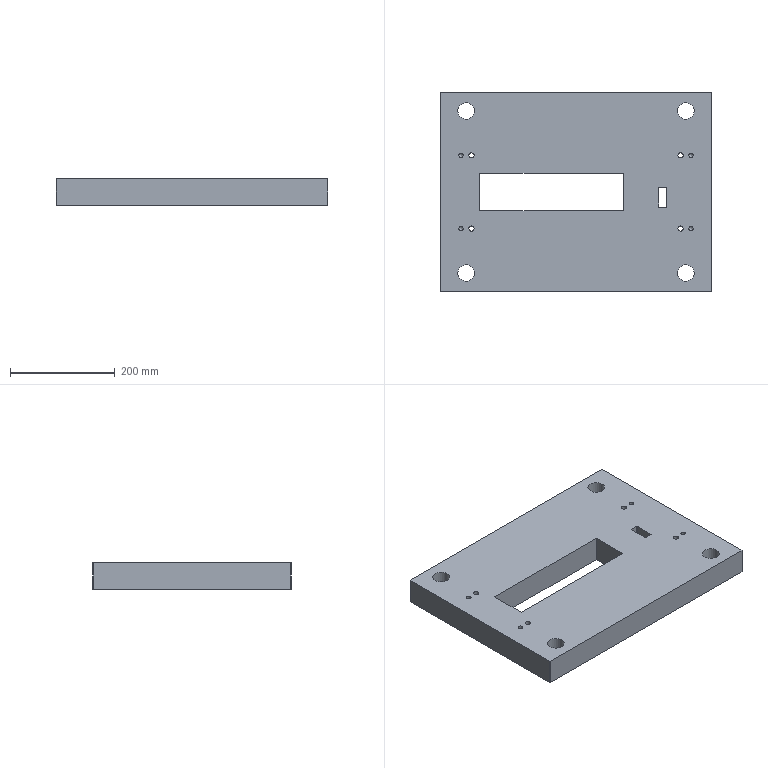Part | NX | features BREP 1 | 1 solid | 58 faces | box 520 x 380 x 50 mm | volume 8655662 mm3 | plane 30 | cylinder 24 | cone 4 | commonest cylinder face diameters 1 x4 8.5 x4 10 x4 10.8 x4 32 x4 40.5 x4
STEP:
#1=CARTESIAN_POINT('',(-184.123,-36.004,-90.6));
#2=VERTEX_POINT('',#1);
#3=CARTESIAN_POINT('',(-184.123,36.,-90.6));
#4=VERTEX_POINT('',#3);
#5=CARTESIAN_POINT('',(-184.123,190.,-90.6));
#6=DIRECTION('',(0.,1.,0.));
#7=VECTOR('',#6,1000.);
#8=LINE('',#5,#7);
#9=EDGE_CURVE('',#2,#4,#8,.T.);
#10=ORIENTED_EDGE('',*,*,#9,.F.);
#11=CARTESIAN_POINT('',(91.05,-36.004,-90.6));
#12=VERTEX_POINT('',#11);
#13=CARTESIAN_POINT('',(-260.,-36.004,-90.6));
#14=DIRECTION('',(-1.,0.,0.));
#15=VECTOR('',#14,1000.);
#16=LINE('',#13,#15);
#17=EDGE_CURVE('',#12,#2,#16,.T.);
#18=ORIENTED_EDGE('',*,*,#17,.F.);
#19=CARTESIAN_POINT('',(91.05,36.,-90.6));
#20=VERTEX_POINT('',#19);
#21=CARTESIAN_POINT('',(91.05,190.,-90.6));
#22=DIRECTION('',(0.,-1.,0.));
#23=VECTOR('',#22,1000.);
#24=LINE('',#21,#23);
#25=EDGE_CURVE('',#20,#12,#24,.T.);
#26=ORIENTED_EDGE('',*,*,#25,.F.);
#27=CARTESIAN_POINT('',(-260.,36.,-90.6));
#28=DIRECTION('',(1.,0.,0.));
#29=VECTOR('',#28,1000.);
#30=LINE('',#27,#29);
#31=EDGE_CURVE('',#4,#20,#30,.T.);
#32=ORIENTED_EDGE('',*,*,#31,.F.);
#33=EDGE_LOOP('',(#10,#18,#26,#32));
#34=FACE_BOUND('',#33,.T.);
#35=CARTESIAN_POINT('',(158.935,9.214,-90.6));
#36=VERTEX_POINT('',#35);
#37=CARTESIAN_POINT('',(158.435,8.714,-90.6));
#38=VERTEX_POINT('',#37);
#39=CARTESIAN_POINT('',(158.935,8.714,-90.6));
#40=DIRECTION('',(0.,0.,1.));
#41=DIRECTION('',(1.,0.,0.));
#42=AXIS2_PLACEMENT_3D('',#39,#40,#41);
#43=CIRCLE('',#42,0.5);
#44=EDGE_CURVE('',#36,#38,#43,.T.);
#45=ORIENTED_EDGE('',*,*,#44,.T.);
#46=CARTESIAN_POINT('',(158.435,-29.007,-90.6));
#47=VERTEX_POINT('',#46);
#48=CARTESIAN_POINT('',(158.435,-29.007,-90.6));
#49=DIRECTION('',(0.,1.,0.));
#50=VECTOR('',#49,1000.);
#51=LINE('',#48,#50);
#52=EDGE_CURVE('',#47,#38,#51,.T.);
#53=ORIENTED_EDGE('',*,*,#52,.F.);
#54=CARTESIAN_POINT('',(158.935,-29.507,-90.6));
#55=VERTEX_POINT('',#54);
#56=CARTESIAN_POINT('',(158.935,-29.007,-90.6));
#57=DIRECTION('',(0.,0.,1.));
#58=DIRECTION('',(1.,0.,0.));
#59=AXIS2_PLACEMENT_3D('',#56,#57,#58);
#60=CIRCLE('',#59,0.5);
#61=EDGE_CURVE('',#47,#55,#60,.T.);
#62=ORIENTED_EDGE('',*,*,#61,.T.);
#63=CARTESIAN_POINT('',(173.477,-29.507,-90.6));
#64=VERTEX_POINT('',#63);
#65=CARTESIAN_POINT('',(173.477,-29.507,-90.6));
#66=DIRECTION('',(-1.,0.,0.));
#67=VECTOR('',#66,1000.);
#68=LINE('',#65,#67);
#69=EDGE_CURVE('',#64,#55,#68,.T.);
#70=ORIENTED_EDGE('',*,*,#69,.F.);
#71=CARTESIAN_POINT('',(173.977,-29.007,-90.6));
#72=VERTEX_POINT('',#71);
#73=CARTESIAN_POINT('',(173.477,-29.007,-90.6));
#74=DIRECTION('',(0.,0.,1.));
#75=DIRECTION('',(1.,0.,0.));
#76=AXIS2_PLACEMENT_3D('',#73,#74,#75);
#77=CIRCLE('',#76,0.5);
#78=EDGE_CURVE('',#64,#72,#77,.T.);
#79=ORIENTED_EDGE('',*,*,#78,.T.);
#80=CARTESIAN_POINT('',(173.977,8.714,-90.6));
#81=VERTEX_POINT('',#80);
#82=CARTESIAN_POINT('',(173.977,8.714,-90.6));
#83=DIRECTION('',(0.,-1.,0.));
#84=VECTOR('',#83,1000.);
#85=LINE('',#82,#84);
#86=EDGE_CURVE('',#81,#72,#85,.T.);
#87=ORIENTED_EDGE('',*,*,#86,.F.);
#88=CARTESIAN_POINT('',(173.477,9.214,-90.6));
#89=VERTEX_POINT('',#88);
#90=CARTESIAN_POINT('',(173.477,8.714,-90.6));
#91=DIRECTION('',(0.,0.,1.));
#92=DIRECTION('',(1.,0.,0.));
#93=AXIS2_PLACEMENT_3D('',#90,#91,#92);
#94=CIRCLE('',#93,0.5);
#95=EDGE_CURVE('',#81,#89,#94,.T.);
#96=ORIENTED_EDGE('',*,*,#95,.T.);
#97=CARTESIAN_POINT('',(158.935,9.214,-90.6));
#98=DIRECTION('',(1.,0.,0.));
#99=VECTOR('',#98,1000.);
#100=LINE('',#97,#99);
#101=EDGE_CURVE('',#36,#89,#100,.T.);
#102=ORIENTED_EDGE('',*,*,#101,.F.);
#103=EDGE_LOOP('',(#45,#53,#62,#70,#79,#87,#96,#102));
#104=FACE_BOUND('',#103,.T.);
#105=CARTESIAN_POINT('',(-260.,-189.,-90.6));
#106=VERTEX_POINT('',#105);
#107=CARTESIAN_POINT('',(-260.,189.,-90.6));
#108=VERTEX_POINT('',#107);
#109=CARTESIAN_POINT('',(-260.,-190.,-90.6));
#110=DIRECTION('',(0.,1.,0.));
#111=VECTOR('',#110,1000.);
#112=LINE('',#109,#111);
#113=EDGE_CURVE('',#106,#108,#112,.T.);
#114=ORIENTED_EDGE('',*,*,#113,.T.);
#115=CARTESIAN_POINT('',(-259.,190.,-90.6));
#116=VERTEX_POINT('',#115);
#117=CARTESIAN_POINT('',(-259.5,189.5,-90.6));
#118=DIRECTION('',(0.7071,0.7071,0.));
#119=VECTOR('',#118,1000.);
#120=LINE('',#117,#119);
#121=EDGE_CURVE('',#108,#116,#120,.T.);
#122=ORIENTED_EDGE('',*,*,#121,.T.);
#123=CARTESIAN_POINT('',(259.,190.,-90.6));
#124=VERTEX_POINT('',#123);
#125=CARTESIAN_POINT('',(-260.,190.,-90.6));
#126=DIRECTION('',(1.,0.,0.));
#127=VECTOR('',#126,1000.);
#128=LINE('',#125,#127);
#129=EDGE_CURVE('',#116,#124,#128,.T.);
#130=ORIENTED_EDGE('',*,*,#129,.T.);
#131=CARTESIAN_POINT('',(260.,189.,-90.6));
#132=VERTEX_POINT('',#131);
#133=CARTESIAN_POINT('',(-0.5,449.5,-90.6));
#134=DIRECTION('',(0.7071,-0.7071,0.));
#135=VECTOR('',#134,1000.);
#136=LINE('',#133,#135);
#137=EDGE_CURVE('',#124,#132,#136,.T.);
#138=ORIENTED_EDGE('',*,*,#137,.T.);
#139=CARTESIAN_POINT('',(260.,-189.,-90.6));
#140=VERTEX_POINT('',#139);
#141=CARTESIAN_POINT('',(260.,190.,-90.6));
#142=DIRECTION('',(0.,-1.,0.));
#143=VECTOR('',#142,1000.);
#144=LINE('',#141,#143);
#145=EDGE_CURVE('',#132,#140,#144,.T.);
#146=ORIENTED_EDGE('',*,*,#145,.T.);
#147=CARTESIAN_POINT('',(259.,-190.,-90.6));
#148=VERTEX_POINT('',#147);
#149=CARTESIAN_POINT('',(189.5,-259.5,-90.6));
#150=DIRECTION('',(-0.7071,-0.7071,0.));
#151=VECTOR('',#150,1000.);
#152=LINE('',#149,#151);
#153=EDGE_CURVE('',#140,#148,#152,.T.);
#154=ORIENTED_EDGE('',*,*,#153,.T.);
#155=CARTESIAN_POINT('',(-259.,-190.,-90.6));
#156=VERTEX_POINT('',#155);
#157=CARTESIAN_POINT('',(260.,-190.,-90.6));
#158=DIRECTION('',(-1.,0.,0.));
#159=VECTOR('',#158,1000.);
#160=LINE('',#157,#159);
#161=EDGE_CURVE('',#148,#156,#160,.T.);
#162=ORIENTED_EDGE('',*,*,#161,.T.);
#163=CARTESIAN_POINT('',(-449.5,0.5,-90.6));
#164=DIRECTION('',(-0.7071,0.7071,0.));
#165=VECTOR('',#164,1000.);
#166=LINE('',#163,#165);
#167=EDGE_CURVE('',#156,#106,#166,.T.);
#168=ORIENTED_EDGE('',*,*,#167,.T.);
#169=EDGE_LOOP('',(#114,#122,#130,#138,#146,#154,#162,#168));
#170=FACE_BOUND('',#169,.T.);
#171=CARTESIAN_POINT('',(189.75,155.,-90.6));
#172=VERTEX_POINT('',#171);
#173=CARTESIAN_POINT('',(210.,155.,-90.6));
#174=DIRECTION('',(0.,0.,-1.));
#175=DIRECTION('',(-1.,0.,0.));
#176=AXIS2_PLACEMENT_3D('',#173,#174,#175);
#177=CIRCLE('',#176,20.25);
#178=EDGE_CURVE('',#172,#172,#177,.T.);
#179=ORIENTED_EDGE('',*,*,#178,.F.);
#180=EDGE_LOOP('',(#179));
#181=FACE_BOUND('',#180,.T.);
#182=CARTESIAN_POINT('',(-230.25,155.,-90.6));
#183=VERTEX_POINT('',#182);
#184=CARTESIAN_POINT('',(-210.,155.,-90.6));
#185=DIRECTION('',(0.,0.,-1.));
#186=DIRECTION('',(-1.,0.,0.));
#187=AXIS2_PLACEMENT_3D('',#184,#185,#186);
#188=CIRCLE('',#187,20.25);
#189=EDGE_CURVE('',#183,#183,#188,.T.);
#190=ORIENTED_EDGE('',*,*,#189,.F.);
#191=EDGE_LOOP('',(#190));
#192=FACE_BOUND('',#191,.T.);
#193=CARTESIAN_POINT('',(-230.25,-155.,-90.6));
#194=VERTEX_POINT('',#193);
#195=CARTESIAN_POINT('',(-210.,-155.,-90.6));
#196=DIRECTION('',(0.,0.,-1.));
#197=DIRECTION('',(-1.,0.,0.));
#198=AXIS2_PLACEMENT_3D('',#195,#196,#197);
#199=CIRCLE('',#198,20.25);
#200=EDGE_CURVE('',#194,#194,#199,.T.);
#201=ORIENTED_EDGE('',*,*,#200,.F.);
#202=EDGE_LOOP('',(#201));
#203=FACE_BOUND('',#202,.T.);
#204=CARTESIAN_POINT('',(189.75,-155.,-90.6));
#205=VERTEX_POINT('',#204);
#206=CARTESIAN_POINT('',(210.,-155.,-90.6));
#207=DIRECTION('',(0.,0.,-1.));
#208=DIRECTION('',(-1.,0.,0.));
#209=AXIS2_PLACEMENT_3D('',#206,#207,#208);
#210=CIRCLE('',#209,20.25);
#211=EDGE_CURVE('',#205,#205,#210,.T.);
#212=ORIENTED_EDGE('',*,*,#211,.F.);
#213=EDGE_LOOP('',(#212));
#214=FACE_BOUND('',#213,.T.);
#215=CARTESIAN_POINT('',(195.012,-72.068,-90.6));
#216=VERTEX_POINT('',#215);
#217=CARTESIAN_POINT('',(200.,-70.,-90.6));
#218=DIRECTION('',(0.,0.,-1.));
#219=DIRECTION('',(-0.9237,-0.383,0.));
#220=AXIS2_PLACEMENT_3D('',#217,#218,#219);
#221=CIRCLE('',#220,5.4);
#222=EDGE_CURVE('',#216,#216,#221,.T.);
#223=ORIENTED_EDGE('',*,*,#222,.F.);
#224=EDGE_LOOP('',(#223));
#225=FACE_BOUND('',#224,.T.);
#226=CARTESIAN_POINT('',(195.012,67.932,-90.6));
#227=VERTEX_POINT('',#226);
#228=CARTESIAN_POINT('',(200.,70.,-90.6));
#229=DIRECTION('',(0.,0.,-1.));
#230=DIRECTION('',(-0.9237,-0.383,0.));
#231=AXIS2_PLACEMENT_3D('',#228,#229,#230);
#232=CIRCLE('',#231,5.4);
#233=EDGE_CURVE('',#227,#227,#232,.T.);
#234=ORIENTED_EDGE('',*,*,#233,.F.);
#235=EDGE_LOOP('',(#234));
#236=FACE_BOUND('',#235,.T.);
#237=CARTESIAN_POINT('',(-204.988,-72.068,-90.6));
#238=VERTEX_POINT('',#237);
#239=CARTESIAN_POINT('',(-200.,-70.,-90.6));
#240=DIRECTION('',(0.,0.,-1.));
#241=DIRECTION('',(-0.9237,-0.383,0.));
#242=AXIS2_PLACEMENT_3D('',#239,#240,#241);
#243=CIRCLE('',#242,5.4);
#244=EDGE_CURVE('',#238,#238,#243,.T.);
#245=ORIENTED_EDGE('',*,*,#244,.F.);
#246=EDGE_LOOP('',(#245));
#247=FACE_BOUND('',#246,.T.);
#248=CARTESIAN_POINT('',(-204.988,67.932,-90.6));
#249=VERTEX_POINT('',#248);
#250=CARTESIAN_POINT('',(-200.,70.,-90.6));
#251=DIRECTION('',(0.,0.,-1.));
#252=DIRECTION('',(-0.9237,-0.383,0.));
#253=AXIS2_PLACEMENT_3D('',#250,#251,#252);
#254=CIRCLE('',#253,5.4);
#255=EDGE_CURVE('',#249,#249,#254,.T.);
#256=ORIENTED_EDGE('',*,*,#255,.F.);
#257=EDGE_LOOP('',(#256));
#258=FACE_BOUND('',#257,.T.);
#259=CARTESIAN_POINT('',(-260.,190.,-90.6));
#260=DIRECTION('',(0.,0.,-1.));
#261=DIRECTION('',(1.,0.,0.));
#262=AXIS2_PLACEMENT_3D('',#259,#260,#261);
#263=PLANE('',#262);
#264=ADVANCED_FACE('',(#34,#104,#170,#181,#192,#203,#214,#225,#236,#247,#258),#263,.T.);
#265=CARTESIAN_POINT('',(-184.123,-36.004,-40.6));
#266=VERTEX_POINT('',#265);
#267=CARTESIAN_POINT('',(91.05,-36.004,-40.6));
#268=VERTEX_POINT('',#267);
#269=CARTESIAN_POINT('',(-184.123,-36.004,-40.6));
#270=DIRECTION('',(1.,0.,0.));
#271=VECTOR('',#270,1000.);
#272=LINE('',#269,#271);
#273=EDGE_CURVE('',#266,#268,#272,.T.);
#274=ORIENTED_EDGE('',*,*,#273,.F.);
#275=CARTESIAN_POINT('',(-184.123,36.,-40.6));
#276=VERTEX_POINT('',#275);
#277=CARTESIAN_POINT('',(-184.123,36.,-40.6));
#278=DIRECTION('',(0.,-1.,0.));
#279=VECTOR('',#278,1000.);
#280=LINE('',#277,#279);
#281=EDGE_CURVE('',#276,#266,#280,.T.);
#282=ORIENTED_EDGE('',*,*,#281,.F.);
#283=CARTESIAN_POINT('',(91.05,36.,-40.6));
#284=VERTEX_POINT('',#283);
#285=CARTESIAN_POINT('',(91.05,36.,-40.6));
#286=DIRECTION('',(-1.,0.,0.));
#287=VECTOR('',#286,1000.);
#288=LINE('',#285,#287);
#289=EDGE_CURVE('',#284,#276,#288,.T.);
#290=ORIENTED_EDGE('',*,*,#289,.F.);
#291=CARTESIAN_POINT('',(91.05,-36.004,-40.6));
#292=DIRECTION('',(0.,1.,0.));
#293=VECTOR('',#292,1000.);
#294=LINE('',#291,#293);
#295=EDGE_CURVE('',#268,#284,#294,.T.);
#296=ORIENTED_EDGE('',*,*,#295,.F.);
#297=EDGE_LOOP('',(#274,#282,#290,#296));
#298=FACE_BOUND('',#297,.T.);
#299=CARTESIAN_POINT('',(-195.381,71.915,-40.6));
#300=VERTEX_POINT('',#299);
#301=CARTESIAN_POINT('',(-200.,70.,-40.6));
#302=DIRECTION('',(0.,0.,1.));
#303=DIRECTION('',(0.9237,0.383,0.));
#304=AXIS2_PLACEMENT_3D('',#301,#302,#303);
#305=CIRCLE('',#304,5.);
#306=EDGE_CURVE('',#300,#300,#305,.T.);
#307=ORIENTED_EDGE('',*,*,#306,.F.);
#308=EDGE_LOOP('',(#307));
#309=FACE_BOUND('',#308,.T.);
#310=CARTESIAN_POINT('',(-195.381,-68.085,-40.6));
#311=VERTEX_POINT('',#310);
#312=CARTESIAN_POINT('',(-200.,-70.,-40.6));
#313=DIRECTION('',(0.,0.,1.));
#314=DIRECTION('',(0.9237,0.383,0.));
#315=AXIS2_PLACEMENT_3D('',#312,#313,#314);
#316=CIRCLE('',#315,5.);
#317=EDGE_CURVE('',#311,#311,#316,.T.);
#318=ORIENTED_EDGE('',*,*,#317,.F.);
#319=EDGE_LOOP('',(#318));
#320=FACE_BOUND('',#319,.T.);
#321=CARTESIAN_POINT('',(204.619,71.915,-40.6));
#322=VERTEX_POINT('',#321);
#323=CARTESIAN_POINT('',(200.,70.,-40.6));
#324=DIRECTION('',(0.,0.,1.));
#325=DIRECTION('',(0.9237,0.383,0.));
#326=AXIS2_PLACEMENT_3D('',#323,#324,#325);
#327=CIRCLE('',#326,5.);
#328=EDGE_CURVE('',#322,#322,#327,.T.);
#329=ORIENTED_EDGE('',*,*,#328,.F.);
#330=EDGE_LOOP('',(#329));
#331=FACE_BOUND('',#330,.T.);
#332=CARTESIAN_POINT('',(204.619,-68.085,-40.6));
#333=VERTEX_POINT('',#332);
#334=CARTESIAN_POINT('',(200.,-70.,-40.6));
#335=DIRECTION('',(0.,0.,1.));
#336=DIRECTION('',(0.9237,0.383,0.));
#337=AXIS2_PLACEMENT_3D('',#334,#335,#336);
#338=CIRCLE('',#337,5.);
#339=EDGE_CURVE('',#333,#333,#338,.T.);
#340=ORIENTED_EDGE('',*,*,#339,.F.);
#341=EDGE_LOOP('',(#340));
#342=FACE_BOUND('',#341,.T.);
#343=CARTESIAN_POINT('',(215.75,-70.,-40.6));
#344=VERTEX_POINT('',#343);
#345=CARTESIAN_POINT('',(220.,-70.,-40.6));
#346=DIRECTION('',(0.,0.,1.));
#347=DIRECTION('',(-1.,0.,0.));
#348=AXIS2_PLACEMENT_3D('',#345,#346,#347);
#349=CIRCLE('',#348,4.25);
#350=EDGE_CURVE('',#344,#344,#349,.T.);
#351=ORIENTED_EDGE('',*,*,#350,.F.);
#352=EDGE_LOOP('',(#351));
#353=FACE_BOUND('',#352,.T.);
#354=CARTESIAN_POINT('',(-224.25,70.,-40.6));
#355=VERTEX_POINT('',#354);
#356=CARTESIAN_POINT('',(-220.,70.,-40.6));
#357=DIRECTION('',(0.,0.,1.));
#358=DIRECTION('',(-1.,0.,0.));
#359=AXIS2_PLACEMENT_3D('',#356,#357,#358);
#360=CIRCLE('',#359,4.25);
#361=EDGE_CURVE('',#355,#355,#360,.T.);
#362=ORIENTED_EDGE('',*,*,#361,.F.);
#363=EDGE_LOOP('',(#362));
#364=FACE_BOUND('',#363,.T.);
#365=CARTESIAN_POINT('',(-224.25,-70.,-40.6));
#366=VERTEX_POINT('',#365);
#367=CARTESIAN_POINT('',(-220.,-70.,-40.6));
#368=DIRECTION('',(0.,0.,1.));
#369=DIRECTION('',(-1.,0.,0.));
#370=AXIS2_PLACEMENT_3D('',#367,#368,#369);
#371=CIRCLE('',#370,4.25);
#372=EDGE_CURVE('',#366,#366,#371,.T.);
#373=ORIENTED_EDGE('',*,*,#372,.F.);
#374=EDGE_LOOP('',(#373));
#375=FACE_BOUND('',#374,.T.);
#376=CARTESIAN_POINT('',(215.75,70.,-40.6));
#377=VERTEX_POINT('',#376);
#378=CARTESIAN_POINT('',(220.,70.,-40.6));
#379=DIRECTION('',(0.,0.,1.));
#380=DIRECTION('',(-1.,0.,0.));
#381=AXIS2_PLACEMENT_3D('',#378,#379,#380);
#382=CIRCLE('',#381,4.25);
#383=EDGE_CURVE('',#377,#377,#382,.T.);
#384=ORIENTED_EDGE('',*,*,#383,.F.);
#385=EDGE_LOOP('',(#384));
#386=FACE_BOUND('',#385,.T.);
#387=CARTESIAN_POINT('',(226.,-155.,-40.6));
#388=VERTEX_POINT('',#387);
#389=CARTESIAN_POINT('',(210.,-155.,-40.6));
#390=DIRECTION('',(0.,0.,1.));
#391=DIRECTION('',(1.,0.,0.));
#392=AXIS2_PLACEMENT_3D('',#389,#390,#391);
#393=CIRCLE('',#392,16.);
#394=EDGE_CURVE('',#388,#388,#393,.T.);
#395=ORIENTED_EDGE('',*,*,#394,.F.);
#396=EDGE_LOOP('',(#395));
#397=FACE_BOUND('',#396,.T.);
#398=CARTESIAN_POINT('',(-194.,-155.,-40.6));
#399=VERTEX_POINT('',#398);
#400=CARTESIAN_POINT('',(-210.,-155.,-40.6));
#401=DIRECTION('',(0.,0.,1.));
#402=DIRECTION('',(1.,0.,0.));
#403=AXIS2_PLACEMENT_3D('',#400,#401,#402);
#404=CIRCLE('',#403,16.);
#405=EDGE_CURVE('',#399,#399,#404,.T.);
#406=ORIENTED_EDGE('',*,*,#405,.F.);
#407=EDGE_LOOP('',(#406));
#408=FACE_BOUND('',#407,.T.);
#409=CARTESIAN_POINT('',(-194.,155.,-40.6));
#410=VERTEX_POINT('',#409);
#411=CARTESIAN_POINT('',(-210.,155.,-40.6));
#412=DIRECTION('',(0.,0.,1.));
#413=DIRECTION('',(1.,0.,0.));
#414=AXIS2_PLACEMENT_3D('',#411,#412,#413);
#415=CIRCLE('',#414,16.);
#416=EDGE_CURVE('',#410,#410,#415,.T.);
#417=ORIENTED_EDGE('',*,*,#416,.F.);
#418=EDGE_LOOP('',(#417));
#419=FACE_BOUND('',#418,.T.);
#420=CARTESIAN_POINT('',(226.,155.,-40.6));
#421=VERTEX_POINT('',#420);
#422=CARTESIAN_POINT('',(210.,155.,-40.6));
#423=DIRECTION('',(0.,0.,1.));
#424=DIRECTION('',(1.,0.,0.));
#425=AXIS2_PLACEMENT_3D('',#422,#423,#424);
#426=CIRCLE('',#425,16.);
#427=EDGE_CURVE('',#421,#421,#426,.T.);
#428=ORIENTED_EDGE('',*,*,#427,.F.);
#429=EDGE_LOOP('',(#428));
#430=FACE_BOUND('',#429,.T.);
#431=CARTESIAN_POINT('',(-259.,190.,-40.6));
#432=VERTEX_POINT('',#431);
#433=CARTESIAN_POINT('',(259.,190.,-40.6));
#434=VERTEX_POINT('',#433);
#435=CARTESIAN_POINT('',(-260.,190.,-40.6));
#436=DIRECTION('',(1.,0.,0.));
#437=VECTOR('',#436,1000.);
#438=LINE('',#435,#437);
#439=EDGE_CURVE('',#432,#434,#438,.T.);
#440=ORIENTED_EDGE('',*,*,#439,.F.);
#441=CARTESIAN_POINT('',(-260.,189.,-40.6));
#442=VERTEX_POINT('',#441);
#443=CARTESIAN_POINT('',(-259.,190.,-40.6));
#444=DIRECTION('',(-0.7071,-0.7071,0.));
#445=VECTOR('',#444,1000.);
#446=LINE('',#443,#445);
#447=EDGE_CURVE('',#432,#442,#446,.T.);
#448=ORIENTED_EDGE('',*,*,#447,.T.);
#449=CARTESIAN_POINT('',(-260.,-189.,-40.6));
#450=VERTEX_POINT('',#449);
#451=CARTESIAN_POINT('',(-260.,-190.,-40.6));
#452=DIRECTION('',(0.,1.,0.));
#453=VECTOR('',#452,1000.);
#454=LINE('',#451,#453);
#455=EDGE_CURVE('',#450,#442,#454,.T.);
#456=ORIENTED_EDGE('',*,*,#455,.F.);
#457=CARTESIAN_POINT('',(-259.,-190.,-40.6));
#458=VERTEX_POINT('',#457);
#459=CARTESIAN_POINT('',(-260.,-189.,-40.6));
#460=DIRECTION('',(0.7071,-0.7071,0.));
#461=VECTOR('',#460,1000.);
#462=LINE('',#459,#461);
#463=EDGE_CURVE('',#450,#458,#462,.T.);
#464=ORIENTED_EDGE('',*,*,#463,.T.);
#465=CARTESIAN_POINT('',(259.,-190.,-40.6));
#466=VERTEX_POINT('',#465);
#467=CARTESIAN_POINT('',(260.,-190.,-40.6));
#468=DIRECTION('',(-1.,0.,0.));
#469=VECTOR('',#468,1000.);
#470=LINE('',#467,#469);
#471=EDGE_CURVE('',#466,#458,#470,.T.);
#472=ORIENTED_EDGE('',*,*,#471,.F.);
#473=CARTESIAN_POINT('',(260.,-189.,-40.6));
#474=VERTEX_POINT('',#473);
#475=CARTESIAN_POINT('',(259.,-190.,-40.6));
#476=DIRECTION('',(0.7071,0.7071,0.));
#477=VECTOR('',#476,1000.);
#478=LINE('',#475,#477);
#479=EDGE_CURVE('',#466,#474,#478,.T.);
#480=ORIENTED_EDGE('',*,*,#479,.T.);
#481=CARTESIAN_POINT('',(260.,189.,-40.6));
#482=VERTEX_POINT('',#481);
#483=CARTESIAN_POINT('',(260.,190.,-40.6));
#484=DIRECTION('',(0.,-1.,0.));
#485=VECTOR('',#484,1000.);
#486=LINE('',#483,#485);
#487=EDGE_CURVE('',#482,#474,#486,.T.);
#488=ORIENTED_EDGE('',*,*,#487,.F.);
#489=CARTESIAN_POINT('',(260.,189.,-40.6));
#490=DIRECTION('',(-0.7071,0.7071,0.));
#491=VECTOR('',#490,1000.);
#492=LINE('',#489,#491);
#493=EDGE_CURVE('',#482,#434,#492,.T.);
#494=ORIENTED_EDGE('',*,*,#493,.T.);
#495=EDGE_LOOP('',(#440,#448,#456,#464,#472,#480,#488,#494));
#496=FACE_BOUND('',#495,.T.);
#497=CARTESIAN_POINT('',(158.435,-29.007,-40.6));
#498=VERTEX_POINT('',#497);
#499=CARTESIAN_POINT('',(158.435,8.714,-40.6));
#500=VERTEX_POINT('',#499);
#501=CARTESIAN_POINT('',(158.435,-29.007,-40.6));
#502=DIRECTION('',(0.,1.,0.));
#503=VECTOR('',#502,1000.);
#504=LINE('',#501,#503);
#505=EDGE_CURVE('',#498,#500,#504,.T.);
#506=ORIENTED_EDGE('',*,*,#505,.T.);
#507=CARTESIAN_POINT('',(158.935,9.214,-40.6));
#508=VERTEX_POINT('',#507);
#509=CARTESIAN_POINT('',(158.935,8.714,-40.6));
#510=DIRECTION('',(0.,0.,1.));
#511=DIRECTION('',(1.,0.,0.));
#512=AXIS2_PLACEMENT_3D('',#509,#510,#511);
#513=CIRCLE('',#512,0.5);
#514=EDGE_CURVE('',#508,#500,#513,.T.);
#515=ORIENTED_EDGE('',*,*,#514,.F.);
#516=CARTESIAN_POINT('',(173.477,9.214,-40.6));
#517=VERTEX_POINT('',#516);
#518=CARTESIAN_POINT('',(158.935,9.214,-40.6));
#519=DIRECTION('',(1.,0.,0.));
#520=VECTOR('',#519,1000.);
#521=LINE('',#518,#520);
#522=EDGE_CURVE('',#508,#517,#521,.T.);
#523=ORIENTED_EDGE('',*,*,#522,.T.);
#524=CARTESIAN_POINT('',(173.977,8.714,-40.6));
#525=VERTEX_POINT('',#524);
#526=CARTESIAN_POINT('',(173.477,8.714,-40.6));
#527=DIRECTION('',(0.,0.,1.));
#528=DIRECTION('',(1.,0.,0.));
#529=AXIS2_PLACEMENT_3D('',#526,#527,#528);
#530=CIRCLE('',#529,0.5);
#531=EDGE_CURVE('',#525,#517,#530,.T.);
#532=ORIENTED_EDGE('',*,*,#531,.F.);
#533=CARTESIAN_POINT('',(173.977,-29.007,-40.6));
#534=VERTEX_POINT('',#533);
#535=CARTESIAN_POINT('',(173.977,8.714,-40.6));
#536=DIRECTION('',(0.,-1.,0.));
#537=VECTOR('',#536,1000.);
#538=LINE('',#535,#537);
#539=EDGE_CURVE('',#525,#534,#538,.T.);
#540=ORIENTED_EDGE('',*,*,#539,.T.);
#541=CARTESIAN_POINT('',(173.477,-29.507,-40.6));
#542=VERTEX_POINT('',#541);
#543=CARTESIAN_POINT('',(173.477,-29.007,-40.6));
#544=DIRECTION('',(0.,0.,1.));
#545=DIRECTION('',(1.,0.,0.));
#546=AXIS2_PLACEMENT_3D('',#543,#544,#545);
#547=CIRCLE('',#546,0.5);
#548=EDGE_CURVE('',#542,#534,#547,.T.);
#549=ORIENTED_EDGE('',*,*,#548,.F.);
#550=CARTESIAN_POINT('',(158.935,-29.507,-40.6));
#551=VERTEX_POINT('',#550);
#552=CARTESIAN_POINT('',(173.477,-29.507,-40.6));
#553=DIRECTION('',(-1.,0.,0.));
#554=VECTOR('',#553,1000.);
#555=LINE('',#552,#554);
#556=EDGE_CURVE('',#542,#551,#555,.T.);
#557=ORIENTED_EDGE('',*,*,#556,.T.);
#558=CARTESIAN_POINT('',(158.935,-29.007,-40.6));
#559=DIRECTION('',(0.,0.,1.));
#560=DIRECTION('',(1.,0.,0.));
#561=AXIS2_PLACEMENT_3D('',#558,#559,#560);
#562=CIRCLE('',#561,0.5);
#563=EDGE_CURVE('',#498,#551,#562,.T.);
#564=ORIENTED_EDGE('',*,*,#563,.F.);
#565=EDGE_LOOP('',(#506,#515,#523,#532,#540,#549,#557,#564));
#566=FACE_BOUND('',#565,.T.);
#567=CARTESIAN_POINT('',(-260.,190.,-40.6));
#568=DIRECTION('',(0.,0.,-1.));
#569=DIRECTION('',(1.,0.,0.));
#570=AXIS2_PLACEMENT_3D('',#567,#568,#569);
#571=PLANE('',#570);
#572=ADVANCED_FACE('',(#298,#309,#320,#331,#342,#353,#364,#375,#386,#397,#408,#419,#430,#496,#566),#571,.F.);
#573=ORIENTED_EDGE('',*,*,#455,.T.);
#574=CARTESIAN_POINT('',(-260.,189.,-90.6));
#575=DIRECTION('',(0.,0.,-1.));
#576=VECTOR('',#575,1000.);
#577=LINE('',#574,#576);
#578=EDGE_CURVE('',#442,#108,#577,.T.);
#579=ORIENTED_EDGE('',*,*,#578,.T.);
#580=ORIENTED_EDGE('',*,*,#113,.F.);
#581=CARTESIAN_POINT('',(-260.,-189.,-90.6));
#582=DIRECTION('',(0.,0.,1.));
#583=VECTOR('',#582,1000.);
#584=LINE('',#581,#583);
#585=EDGE_CURVE('',#106,#450,#584,.T.);
#586=ORIENTED_EDGE('',*,*,#585,.T.);
#587=EDGE_LOOP('',(#573,#579,#580,#586));
#588=FACE_BOUND('',#587,.T.);
#589=CARTESIAN_POINT('',(-260.,-190.,-90.6));
#590=DIRECTION('',(1.,0.,0.));
#591=DIRECTION('',(0.,0.,1.));
#592=AXIS2_PLACEMENT_3D('',#589,#590,#591);
#593=PLANE('',#592);
#594=ADVANCED_FACE('',(#588),#593,.F.);
#595=ORIENTED_EDGE('',*,*,#129,.F.);
#596=CARTESIAN_POINT('',(-259.,190.,-90.6));
#597=DIRECTION('',(0.,0.,1.));
#598=VECTOR('',#597,1000.);
#599=LINE('',#596,#598);
#600=EDGE_CURVE('',#116,#432,#599,.T.);
#601=ORIENTED_EDGE('',*,*,#600,.T.);
#602=ORIENTED_EDGE('',*,*,#439,.T.);
#603=CARTESIAN_POINT('',(259.,190.,-90.6));
#604=DIRECTION('',(0.,0.,-1.));
#605=VECTOR('',#604,1000.);
#606=LINE('',#603,#605);
#607=EDGE_CURVE('',#434,#124,#606,.T.);
#608=ORIENTED_EDGE('',*,*,#607,.T.);
#609=EDGE_LOOP('',(#595,#601,#602,#608));
#610=FACE_BOUND('',#609,.T.);
#611=CARTESIAN_POINT('',(-260.,190.,-90.6));
#612=DIRECTION('',(0.,-1.,0.));
#613=DIRECTION('',(0.,0.,1.));
#614=AXIS2_PLACEMENT_3D('',#611,#612,#613);
#615=PLANE('',#614);
#616=ADVANCED_FACE('',(#610),#615,.F.);
#617=ORIENTED_EDGE('',*,*,#145,.F.);
#618=CARTESIAN_POINT('',(260.,189.,-90.6));
#619=DIRECTION('',(0.,0.,1.));
#620=VECTOR('',#619,1000.);
#621=LINE('',#618,#620);
#622=EDGE_CURVE('',#132,#482,#621,.T.);
#623=ORIENTED_EDGE('',*,*,#622,.T.);
#624=ORIENTED_EDGE('',*,*,#487,.T.);
#625=CARTESIAN_POINT('',(260.,-189.,-90.6));
#626=DIRECTION('',(0.,0.,-1.));
#627=VECTOR('',#626,1000.);
#628=LINE('',#625,#627);
#629=EDGE_CURVE('',#474,#140,#628,.T.);
#630=ORIENTED_EDGE('',*,*,#629,.T.);
#631=EDGE_LOOP('',(#617,#623,#624,#630));
#632=FACE_BOUND('',#631,.T.);
#633=CARTESIAN_POINT('',(260.,190.,-90.6));
#634=DIRECTION('',(-1.,0.,0.));
#635=DIRECTION('',(0.,0.,-1.));
#636=AXIS2_PLACEMENT_3D('',#633,#634,#635);
#637=PLANE('',#636);
#638=ADVANCED_FACE('',(#632),#637,.F.);
#639=ORIENTED_EDGE('',*,*,#161,.F.);
#640=CARTESIAN_POINT('',(259.,-190.,-90.6));
#641=DIRECTION('',(0.,0.,1.));
#642=VECTOR('',#641,1000.);
#643=LINE('',#640,#642);
#644=EDGE_CURVE('',#148,#466,#643,.T.);
#645=ORIENTED_EDGE('',*,*,#644,.T.);
#646=ORIENTED_EDGE('',*,*,#471,.T.);
#647=CARTESIAN_POINT('',(-259.,-190.,-90.6));
#648=DIRECTION('',(0.,0.,-1.));
#649=VECTOR('',#648,1000.);
#650=LINE('',#647,#649);
#651=EDGE_CURVE('',#458,#156,#650,.T.);
#652=ORIENTED_EDGE('',*,*,#651,.T.);
#653=EDGE_LOOP('',(#639,#645,#646,#652));
#654=FACE_BOUND('',#653,.T.);
#655=CARTESIAN_POINT('',(260.,-190.,-90.6));
#656=DIRECTION('',(0.,1.,0.));
#657=DIRECTION('',(1.,0.,0.));
#658=AXIS2_PLACEMENT_3D('',#655,#656,#657);
#659=PLANE('',#658);
#660=ADVANCED_FACE('',(#654),#659,.F.);
#661=ORIENTED_EDGE('',*,*,#121,.F.);
#662=ORIENTED_EDGE('',*,*,#578,.F.);
#663=ORIENTED_EDGE('',*,*,#447,.F.);
#664=ORIENTED_EDGE('',*,*,#600,.F.);
#665=EDGE_LOOP('',(#661,#662,#663,#664));
#666=FACE_BOUND('',#665,.T.);
#667=CARTESIAN_POINT('',(-259.,190.,-90.6));
#668=DIRECTION('',(0.7071,-0.7071,0.));
#669=DIRECTION('',(-0.7071,-0.7071,0.));
#670=AXIS2_PLACEMENT_3D('',#667,#668,#669);
#671=PLANE('',#670);
#672=ADVANCED_FACE('',(#666),#671,.F.);
#673=ORIENTED_EDGE('',*,*,#137,.F.);
#674=ORIENTED_EDGE('',*,*,#607,.F.);
#675=ORIENTED_EDGE('',*,*,#493,.F.);
#676=ORIENTED_EDGE('',*,*,#622,.F.);
#677=EDGE_LOOP('',(#673,#674,#675,#676));
#678=FACE_BOUND('',#677,.T.);
#679=CARTESIAN_POINT('',(260.,189.,-90.6));
#680=DIRECTION('',(-0.7071,-0.7071,0.));
#681=DIRECTION('',(-0.7071,0.7071,0.));
#682=AXIS2_PLACEMENT_3D('',#679,#680,#681);
#683=PLANE('',#682);
#684=ADVANCED_FACE('',(#678),#683,.F.);
#685=ORIENTED_EDGE('',*,*,#153,.F.);
#686=ORIENTED_EDGE('',*,*,#629,.F.);
#687=ORIENTED_EDGE('',*,*,#479,.F.);
#688=ORIENTED_EDGE('',*,*,#644,.F.);
#689=EDGE_LOOP('',(#685,#686,#687,#688));
#690=FACE_BOUND('',#689,.T.);
#691=CARTESIAN_POINT('',(259.,-190.,-90.6));
#692=DIRECTION('',(-0.7071,0.7071,0.));
#693=DIRECTION('',(0.7071,0.7071,0.));
#694=AXIS2_PLACEMENT_3D('',#691,#692,#693);
#695=PLANE('',#694);
#696=ADVANCED_FACE('',(#690),#695,.F.);
#697=ORIENTED_EDGE('',*,*,#167,.F.);
#698=ORIENTED_EDGE('',*,*,#651,.F.);
#699=ORIENTED_EDGE('',*,*,#463,.F.);
#700=ORIENTED_EDGE('',*,*,#585,.F.);
#701=EDGE_LOOP('',(#697,#698,#699,#700));
#702=FACE_BOUND('',#701,.T.);
#703=CARTESIAN_POINT('',(-260.,-189.,-90.6));
#704=DIRECTION('',(0.7071,0.7071,0.));
#705=DIRECTION('',(0.7071,-0.7071,0.));
#706=AXIS2_PLACEMENT_3D('',#703,#704,#705);
#707=PLANE('',#706);
#708=ADVANCED_FACE('',(#702),#707,.F.);
#709=ORIENTED_EDGE('',*,*,#427,.T.);
#710=EDGE_LOOP('',(#709));
#711=FACE_BOUND('',#710,.T.);
#712=CARTESIAN_POINT('',(194.,155.,-79.6));
#713=VERTEX_POINT('',#712);
#714=CARTESIAN_POINT('',(210.,155.,-79.6));
#715=DIRECTION('',(0.,0.,1.));
#716=DIRECTION('',(-1.,0.,0.));
#717=AXIS2_PLACEMENT_3D('',#714,#715,#716);
#718=CIRCLE('',#717,16.);
#719=EDGE_CURVE('',#713,#713,#718,.T.);
#720=ORIENTED_EDGE('',*,*,#719,.F.);
#721=EDGE_LOOP('',(#720));
#722=FACE_BOUND('',#721,.T.);
#723=CARTESIAN_POINT('',(210.,155.,-63.6));
#724=DIRECTION('',(0.,0.,1.));
#725=DIRECTION('',(-1.,0.,0.));
#726=AXIS2_PLACEMENT_3D('',#723,#724,#725);
#727=CYLINDRICAL_SURFACE('',#726,16.);
#728=ADVANCED_FACE('',(#711,#722),#727,.F.);
#729=ORIENTED_EDGE('',*,*,#719,.T.);
#730=EDGE_LOOP('',(#729));
#731=FACE_BOUND('',#730,.T.);
#732=CARTESIAN_POINT('',(189.75,155.,-79.6));
#733=VERTEX_POINT('',#732);
#734=CARTESIAN_POINT('',(210.,155.,-79.6));
#735=DIRECTION('',(0.,0.,1.));
#736=DIRECTION('',(-1.,0.,0.));
#737=AXIS2_PLACEMENT_3D('',#734,#735,#736);
#738=CIRCLE('',#737,20.25);
#739=EDGE_CURVE('',#733,#733,#738,.T.);
#740=ORIENTED_EDGE('',*,*,#739,.F.);
#741=EDGE_LOOP('',(#740));
#742=FACE_BOUND('',#741,.T.);
#743=CARTESIAN_POINT('',(210.,155.,-79.6));
#744=DIRECTION('',(0.,0.,1.));
#745=DIRECTION('',(-1.,0.,0.));
#746=AXIS2_PLACEMENT_3D('',#743,#744,#745);
#747=PLANE('',#746);
#748=ADVANCED_FACE('',(#731,#742),#747,.F.);
#749=ORIENTED_EDGE('',*,*,#178,.T.);
#750=EDGE_LOOP('',(#749));
#751=FACE_BOUND('',#750,.T.);
#752=ORIENTED_EDGE('',*,*,#739,.T.);
#753=EDGE_LOOP('',(#752));
#754=FACE_BOUND('',#753,.T.);
#755=CARTESIAN_POINT('',(210.,155.,-79.6));
#756=DIRECTION('',(0.,0.,-1.));
#757=DIRECTION('',(1.,0.,0.));
#758=AXIS2_PLACEMENT_3D('',#755,#756,#757);
#759=CYLINDRICAL_SURFACE('',#758,20.25);
#760=ADVANCED_FACE('',(#751,#754),#759,.F.);
#761=ORIENTED_EDGE('',*,*,#416,.T.);
#762=EDGE_LOOP('',(#761));
#763=FACE_BOUND('',#762,.T.);
#764=CARTESIAN_POINT('',(-226.,155.,-79.6));
#765=VERTEX_POINT('',#764);
#766=CARTESIAN_POINT('',(-210.,155.,-79.6));
#767=DIRECTION('',(0.,0.,1.));
#768=DIRECTION('',(-1.,0.,0.));
#769=AXIS2_PLACEMENT_3D('',#766,#767,#768);
#770=CIRCLE('',#769,16.);
#771=EDGE_CURVE('',#765,#765,#770,.T.);
#772=ORIENTED_EDGE('',*,*,#771,.F.);
#773=EDGE_LOOP('',(#772));
#774=FACE_BOUND('',#773,.T.);
#775=CARTESIAN_POINT('',(-210.,155.,-63.6));
#776=DIRECTION('',(0.,0.,1.));
#777=DIRECTION('',(-1.,0.,0.));
#778=AXIS2_PLACEMENT_3D('',#775,#776,#777);
#779=CYLINDRICAL_SURFACE('',#778,16.);
#780=ADVANCED_FACE('',(#763,#774),#779,.F.);
#781=ORIENTED_EDGE('',*,*,#771,.T.);
#782=EDGE_LOOP('',(#781));
#783=FACE_BOUND('',#782,.T.);
#784=CARTESIAN_POINT('',(-230.25,155.,-79.6));
#785=VERTEX_POINT('',#784);
#786=CARTESIAN_POINT('',(-210.,155.,-79.6));
#787=DIRECTION('',(0.,0.,1.));
#788=DIRECTION('',(-1.,0.,0.));
#789=AXIS2_PLACEMENT_3D('',#786,#787,#788);
#790=CIRCLE('',#789,20.25);
#791=EDGE_CURVE('',#785,#785,#790,.T.);
#792=ORIENTED_EDGE('',*,*,#791,.F.);
#793=EDGE_LOOP('',(#792));
#794=FACE_BOUND('',#793,.T.);
#795=CARTESIAN_POINT('',(-210.,155.,-79.6));
#796=DIRECTION('',(0.,0.,1.));
#797=DIRECTION('',(-1.,0.,0.));
#798=AXIS2_PLACEMENT_3D('',#795,#796,#797);
#799=PLANE('',#798);
#800=ADVANCED_FACE('',(#783,#794),#799,.F.);
#801=ORIENTED_EDGE('',*,*,#189,.T.);
#802=EDGE_LOOP('',(#801));
#803=FACE_BOUND('',#802,.T.);
#804=ORIENTED_EDGE('',*,*,#791,.T.);
#805=EDGE_LOOP('',(#804));
#806=FACE_BOUND('',#805,.T.);
#807=CARTESIAN_POINT('',(-210.,155.,-79.6));
#808=DIRECTION('',(0.,0.,-1.));
#809=DIRECTION('',(1.,0.,0.));
#810=AXIS2_PLACEMENT_3D('',#807,#808,#809);
#811=CYLINDRICAL_SURFACE('',#810,20.25);
#812=ADVANCED_FACE('',(#803,#806),#811,.F.);
#813=ORIENTED_EDGE('',*,*,#405,.T.);
#814=EDGE_LOOP('',(#813));
#815=FACE_BOUND('',#814,.T.);
#816=CARTESIAN_POINT('',(-226.,-155.,-79.6));
#817=VERTEX_POINT('',#816);
#818=CARTESIAN_POINT('',(-210.,-155.,-79.6));
#819=DIRECTION('',(0.,0.,1.));
#820=DIRECTION('',(-1.,0.,0.));
#821=AXIS2_PLACEMENT_3D('',#818,#819,#820);
#822=CIRCLE('',#821,16.);
#823=EDGE_CURVE('',#817,#817,#822,.T.);
#824=ORIENTED_EDGE('',*,*,#823,.F.);
#825=EDGE_LOOP('',(#824));
#826=FACE_BOUND('',#825,.T.);
#827=CARTESIAN_POINT('',(-210.,-155.,-63.6));
#828=DIRECTION('',(0.,0.,1.));
#829=DIRECTION('',(-1.,0.,0.));
#830=AXIS2_PLACEMENT_3D('',#827,#828,#829);
#831=CYLINDRICAL_SURFACE('',#830,16.);
#832=ADVANCED_FACE('',(#815,#826),#831,.F.);
#833=ORIENTED_EDGE('',*,*,#823,.T.);
#834=EDGE_LOOP('',(#833));
#835=FACE_BOUND('',#834,.T.);
#836=CARTESIAN_POINT('',(-230.25,-155.,-79.6));
#837=VERTEX_POINT('',#836);
#838=CARTESIAN_POINT('',(-210.,-155.,-79.6));
#839=DIRECTION('',(0.,0.,1.));
#840=DIRECTION('',(-1.,0.,0.));
#841=AXIS2_PLACEMENT_3D('',#838,#839,#840);
#842=CIRCLE('',#841,20.25);
#843=EDGE_CURVE('',#837,#837,#842,.T.);
#844=ORIENTED_EDGE('',*,*,#843,.F.);
#845=EDGE_LOOP('',(#844));
#846=FACE_BOUND('',#845,.T.);
#847=CARTESIAN_POINT('',(-210.,-155.,-79.6));
#848=DIRECTION('',(0.,0.,1.));
#849=DIRECTION('',(-1.,0.,0.));
#850=AXIS2_PLACEMENT_3D('',#847,#848,#849);
#851=PLANE('',#850);
#852=ADVANCED_FACE('',(#835,#846),#851,.F.);
#853=ORIENTED_EDGE('',*,*,#200,.T.);
#854=EDGE_LOOP('',(#853));
#855=FACE_BOUND('',#854,.T.);
#856=ORIENTED_EDGE('',*,*,#843,.T.);
#857=EDGE_LOOP('',(#856));
#858=FACE_BOUND('',#857,.T.);
#859=CARTESIAN_POINT('',(-210.,-155.,-79.6));
#860=DIRECTION('',(0.,0.,-1.));
#861=DIRECTION('',(1.,0.,0.));
#862=AXIS2_PLACEMENT_3D('',#859,#860,#861);
#863=CYLINDRICAL_SURFACE('',#862,20.25);
#864=ADVANCED_FACE('',(#855,#858),#863,.F.);
#865=ORIENTED_EDGE('',*,*,#394,.T.);
#866=EDGE_LOOP('',(#865));
#867=FACE_BOUND('',#866,.T.);
#868=CARTESIAN_POINT('',(194.,-155.,-79.6));
#869=VERTEX_POINT('',#868);
#870=CARTESIAN_POINT('',(210.,-155.,-79.6));
#871=DIRECTION('',(0.,0.,1.));
#872=DIRECTION('',(-1.,0.,0.));
#873=AXIS2_PLACEMENT_3D('',#870,#871,#872);
#874=CIRCLE('',#873,16.);
#875=EDGE_CURVE('',#869,#869,#874,.T.);
#876=ORIENTED_EDGE('',*,*,#875,.F.);
#877=EDGE_LOOP('',(#876));
#878=FACE_BOUND('',#877,.T.);
#879=CARTESIAN_POINT('',(210.,-155.,-63.6));
#880=DIRECTION('',(0.,0.,1.));
#881=DIRECTION('',(-1.,0.,0.));
#882=AXIS2_PLACEMENT_3D('',#879,#880,#881);
#883=CYLINDRICAL_SURFACE('',#882,16.);
#884=ADVANCED_FACE('',(#867,#878),#883,.F.);
#885=ORIENTED_EDGE('',*,*,#875,.T.);
#886=EDGE_LOOP('',(#885));
#887=FACE_BOUND('',#886,.T.);
#888=CARTESIAN_POINT('',(189.75,-155.,-79.6));
#889=VERTEX_POINT('',#888);
#890=CARTESIAN_POINT('',(210.,-155.,-79.6));
#891=DIRECTION('',(0.,0.,1.));
#892=DIRECTION('',(-1.,0.,0.));
#893=AXIS2_PLACEMENT_3D('',#890,#891,#892);
#894=CIRCLE('',#893,20.25);
#895=EDGE_CURVE('',#889,#889,#894,.T.);
#896=ORIENTED_EDGE('',*,*,#895,.F.);
#897=EDGE_LOOP('',(#896));
#898=FACE_BOUND('',#897,.T.);
#899=CARTESIAN_POINT('',(210.,-155.,-79.6));
#900=DIRECTION('',(0.,0.,1.));
#901=DIRECTION('',(-1.,0.,0.));
#902=AXIS2_PLACEMENT_3D('',#899,#900,#901);
#903=PLANE('',#902);
#904=ADVANCED_FACE('',(#887,#898),#903,.F.);
#905=ORIENTED_EDGE('',*,*,#211,.T.);
#906=EDGE_LOOP('',(#905));
#907=FACE_BOUND('',#906,.T.);
#908=ORIENTED_EDGE('',*,*,#895,.T.);
#909=EDGE_LOOP('',(#908));
#910=FACE_BOUND('',#909,.T.);
#911=CARTESIAN_POINT('',(210.,-155.,-79.6));
#912=DIRECTION('',(0.,0.,-1.));
#913=DIRECTION('',(1.,0.,0.));
#914=AXIS2_PLACEMENT_3D('',#911,#912,#913);
#915=CYLINDRICAL_SURFACE('',#914,20.25);
#916=ADVANCED_FACE('',(#907,#910),#915,.F.);
#917=ORIENTED_EDGE('',*,*,#383,.T.);
#918=EDGE_LOOP('',(#917));
#919=FACE_BOUND('',#918,.T.);
#920=CARTESIAN_POINT('',(215.75,70.,-63.4));
#921=VERTEX_POINT('',#920);
#922=CARTESIAN_POINT('',(220.,70.,-63.4));
#923=DIRECTION('',(0.,0.,1.));
#924=DIRECTION('',(-1.,0.,0.));
#925=AXIS2_PLACEMENT_3D('',#922,#923,#924);
#926=CIRCLE('',#925,4.25);
#927=EDGE_CURVE('',#921,#921,#926,.T.);
#928=ORIENTED_EDGE('',*,*,#927,.F.);
#929=EDGE_LOOP('',(#928));
#930=FACE_BOUND('',#929,.T.);
#931=CARTESIAN_POINT('',(220.,70.,-63.4));
#932=DIRECTION('',(0.,0.,1.));
#933=DIRECTION('',(-1.,0.,0.));
#934=AXIS2_PLACEMENT_3D('',#931,#932,#933);
#935=CYLINDRICAL_SURFACE('',#934,4.25);
#936=ADVANCED_FACE('',(#919,#930),#935,.F.);
#937=CARTESIAN_POINT('',(219.797,70.,-65.831));
#938=VERTEX_POINT('',#937);
#939=CARTESIAN_POINT('',(220.,70.,-65.831));
#940=DIRECTION('',(0.,0.,1.));
#941=DIRECTION('',(-1.,0.,0.));
#942=AXIS2_PLACEMENT_3D('',#939,#940,#941);
#943=CIRCLE('',#942,0.2034);
#944=EDGE_CURVE('',#938,#938,#943,.T.);
#945=ORIENTED_EDGE('',*,*,#944,.T.);
#946=EDGE_LOOP('',(#945));
#947=FACE_BOUND('',#946,.T.);
#948=CARTESIAN_POINT('',(220.,70.,-65.831));
#949=DIRECTION('',(0.,0.,-1.));
#950=DIRECTION('',(1.,0.,0.));
#951=AXIS2_PLACEMENT_3D('',#948,#949,#950);
#952=PLANE('',#951);
#953=ADVANCED_FACE('',(#947),#952,.F.);
#954=ORIENTED_EDGE('',*,*,#944,.F.);
#955=EDGE_LOOP('',(#954));
#956=FACE_BOUND('',#955,.T.);
#957=ORIENTED_EDGE('',*,*,#927,.T.);
#958=EDGE_LOOP('',(#957));
#959=FACE_BOUND('',#958,.T.);
#960=CARTESIAN_POINT('',(220.,70.,-63.4));
#961=DIRECTION('',(0.,0.,1.));
#962=DIRECTION('',(-1.,0.,0.));
#963=AXIS2_PLACEMENT_3D('',#960,#961,#962);
#964=CONICAL_SURFACE('',#963,4.25,1.03);
#965=ADVANCED_FACE('',(#956,#959),#964,.F.);
#966=ORIENTED_EDGE('',*,*,#372,.T.);
#967=EDGE_LOOP('',(#966));
#968=FACE_BOUND('',#967,.T.);
#969=CARTESIAN_POINT('',(-224.25,-70.,-63.4));
#970=VERTEX_POINT('',#969);
#971=CARTESIAN_POINT('',(-220.,-70.,-63.4));
#972=DIRECTION('',(0.,0.,1.));
#973=DIRECTION('',(-1.,0.,0.));
#974=AXIS2_PLACEMENT_3D('',#971,#972,#973);
#975=CIRCLE('',#974,4.25);
#976=EDGE_CURVE('',#970,#970,#975,.T.);
#977=ORIENTED_EDGE('',*,*,#976,.F.);
#978=EDGE_LOOP('',(#977));
#979=FACE_BOUND('',#978,.T.);
#980=CARTESIAN_POINT('',(-220.,-70.,-63.4));
#981=DIRECTION('',(0.,0.,1.));
#982=DIRECTION('',(-1.,0.,0.));
#983=AXIS2_PLACEMENT_3D('',#980,#981,#982);
#984=CYLINDRICAL_SURFACE('',#983,4.25);
#985=ADVANCED_FACE('',(#968,#979),#984,.F.);
#986=CARTESIAN_POINT('',(-220.203,-70.,-65.831));
#987=VERTEX_POINT('',#986);
#988=CARTESIAN_POINT('',(-220.,-70.,-65.831));
#989=DIRECTION('',(0.,0.,1.));
#990=DIRECTION('',(-1.,0.,0.));
#991=AXIS2_PLACEMENT_3D('',#988,#989,#990);
#992=CIRCLE('',#991,0.2034);
#993=EDGE_CURVE('',#987,#987,#992,.T.);
#994=ORIENTED_EDGE('',*,*,#993,.T.);
#995=EDGE_LOOP('',(#994));
#996=FACE_BOUND('',#995,.T.);
#997=CARTESIAN_POINT('',(-220.,-70.,-65.831));
#998=DIRECTION('',(0.,0.,-1.));
#999=DIRECTION('',(1.,0.,0.));
#1000=AXIS2_PLACEMENT_3D('',#997,#998,#999);
#1001=PLANE('',#1000);
#1002=ADVANCED_FACE('',(#996),#1001,.F.);
#1003=ORIENTED_EDGE('',*,*,#993,.F.);
#1004=EDGE_LOOP('',(#1003));
#1005=FACE_BOUND('',#1004,.T.);
#1006=ORIENTED_EDGE('',*,*,#976,.T.);
#1007=EDGE_LOOP('',(#1006));
#1008=FACE_BOUND('',#1007,.T.);
#1009=CARTESIAN_POINT('',(-220.,-70.,-63.4));
#1010=DIRECTION('',(0.,0.,1.));
#1011=DIRECTION('',(-1.,0.,0.));
#1012=AXIS2_PLACEMENT_3D('',#1009,#1010,#1011);
#1013=CONICAL_SURFACE('',#1012,4.25,1.03);
#1014=ADVANCED_FACE('',(#1005,#1008),#1013,.F.);
#1015=ORIENTED_EDGE('',*,*,#361,.T.);
#1016=EDGE_LOOP('',(#1015));
#1017=FACE_BOUND('',#1016,.T.);
#1018=CARTESIAN_POINT('',(-224.25,70.,-63.4));
#1019=VERTEX_POINT('',#1018);
#1020=CARTESIAN_POINT('',(-220.,70.,-63.4));
#1021=DIRECTION('',(0.,0.,1.));
#1022=DIRECTION('',(-1.,0.,0.));
#1023=AXIS2_PLACEMENT_3D('',#1020,#1021,#1022);
#1024=CIRCLE('',#1023,4.25);
#1025=EDGE_CURVE('',#1019,#1019,#1024,.T.);
#1026=ORIENTED_EDGE('',*,*,#1025,.F.);
#1027=EDGE_LOOP('',(#1026));
#1028=FACE_BOUND('',#1027,.T.);
#1029=CARTESIAN_POINT('',(-220.,70.,-63.4));
#1030=DIRECTION('',(0.,0.,1.));
#1031=DIRECTION('',(-1.,0.,0.));
#1032=AXIS2_PLACEMENT_3D('',#1029,#1030,#1031);
#1033=CYLINDRICAL_SURFACE('',#1032,4.25);
#1034=ADVANCED_FACE('',(#1017,#1028),#1033,.F.);
#1035=CARTESIAN_POINT('',(-220.203,70.,-65.831));
#1036=VERTEX_POINT('',#1035);
#1037=CARTESIAN_POINT('',(-220.,70.,-65.831));
#1038=DIRECTION('',(0.,0.,1.));
#1039=DIRECTION('',(-1.,0.,0.));
#1040=AXIS2_PLACEMENT_3D('',#1037,#1038,#1039);
#1041=CIRCLE('',#1040,0.2034);
#1042=EDGE_CURVE('',#1036,#1036,#1041,.T.);
#1043=ORIENTED_EDGE('',*,*,#1042,.T.);
#1044=EDGE_LOOP('',(#1043));
#1045=FACE_BOUND('',#1044,.T.);
#1046=CARTESIAN_POINT('',(-220.,70.,-65.831));
#1047=DIRECTION('',(0.,0.,-1.));
#1048=DIRECTION('',(1.,0.,0.));
#1049=AXIS2_PLACEMENT_3D('',#1046,#1047,#1048);
#1050=PLANE('',#1049);
#1051=ADVANCED_FACE('',(#1045),#1050,.F.);
#1052=ORIENTED_EDGE('',*,*,#1042,.F.);
#1053=EDGE_LOOP('',(#1052));
#1054=FACE_BOUND('',#1053,.T.);
#1055=ORIENTED_EDGE('',*,*,#1025,.T.);
#1056=EDGE_LOOP('',(#1055));
#1057=FACE_BOUND('',#1056,.T.);
#1058=CARTESIAN_POINT('',(-220.,70.,-63.4));
#1059=DIRECTION('',(0.,0.,1.));
#1060=DIRECTION('',(-1.,0.,0.));
#1061=AXIS2_PLACEMENT_3D('',#1058,#1059,#1060);
#1062=CONICAL_SURFACE('',#1061,4.25,1.03);
#1063=ADVANCED_FACE('',(#1054,#1057),#1062,.F.);
#1064=ORIENTED_EDGE('',*,*,#350,.T.);
#1065=EDGE_LOOP('',(#1064));
#1066=FACE_BOUND('',#1065,.T.);
#1067=CARTESIAN_POINT('',(215.75,-70.,-63.4));
#1068=VERTEX_POINT('',#1067);
#1069=CARTESIAN_POINT('',(220.,-70.,-63.4));
#1070=DIRECTION('',(0.,0.,1.));
#1071=DIRECTION('',(-1.,0.,0.));
#1072=AXIS2_PLACEMENT_3D('',#1069,#1070,#1071);
#1073=CIRCLE('',#1072,4.25);
#1074=EDGE_CURVE('',#1068,#1068,#1073,.T.);
#1075=ORIENTED_EDGE('',*,*,#1074,.F.);
#1076=EDGE_LOOP('',(#1075));
#1077=FACE_BOUND('',#1076,.T.);
#1078=CARTESIAN_POINT('',(220.,-70.,-63.4));
#1079=DIRECTION('',(0.,0.,1.));
#1080=DIRECTION('',(-1.,0.,0.));
#1081=AXIS2_PLACEMENT_3D('',#1078,#1079,#1080);
#1082=CYLINDRICAL_SURFACE('',#1081,4.25);
#1083=ADVANCED_FACE('',(#1066,#1077),#1082,.F.);
#1084=CARTESIAN_POINT('',(219.797,-70.,-65.831));
#1085=VERTEX_POINT('',#1084);
#1086=CARTESIAN_POINT('',(220.,-70.,-65.831));
#1087=DIRECTION('',(0.,0.,1.));
#1088=DIRECTION('',(-1.,0.,0.));
#1089=AXIS2_PLACEMENT_3D('',#1086,#1087,#1088);
#1090=CIRCLE('',#1089,0.2034);
#1091=EDGE_CURVE('',#1085,#1085,#1090,.T.);
#1092=ORIENTED_EDGE('',*,*,#1091,.T.);
#1093=EDGE_LOOP('',(#1092));
#1094=FACE_BOUND('',#1093,.T.);
#1095=CARTESIAN_POINT('',(220.,-70.,-65.831));
#1096=DIRECTION('',(0.,0.,-1.));
#1097=DIRECTION('',(1.,0.,0.));
#1098=AXIS2_PLACEMENT_3D('',#1095,#1096,#1097);
#1099=PLANE('',#1098);
#1100=ADVANCED_FACE('',(#1094),#1099,.F.);
#1101=ORIENTED_EDGE('',*,*,#1091,.F.);
#1102=EDGE_LOOP('',(#1101));
#1103=FACE_BOUND('',#1102,.T.);
#1104=ORIENTED_EDGE('',*,*,#1074,.T.);
#1105=EDGE_LOOP('',(#1104));
#1106=FACE_BOUND('',#1105,.T.);
#1107=CARTESIAN_POINT('',(220.,-70.,-63.4));
#1108=DIRECTION('',(0.,0.,1.));
#1109=DIRECTION('',(-1.,0.,0.));
#1110=AXIS2_PLACEMENT_3D('',#1107,#1108,#1109);
#1111=CONICAL_SURFACE('',#1110,4.25,1.03);
#1112=ADVANCED_FACE('',(#1103,#1106),#1111,.F.);
#1113=CARTESIAN_POINT('',(195.012,-72.068,-85.6));
#1114=VERTEX_POINT('',#1113);
#1115=CARTESIAN_POINT('',(200.,-70.,-85.6));
#1116=DIRECTION('',(0.,0.,1.));
#1117=DIRECTION('',(-0.9237,-0.383,0.));
#1118=AXIS2_PLACEMENT_3D('',#1115,#1116,#1117);
#1119=CIRCLE('',#1118,5.4);
#1120=EDGE_CURVE('',#1114,#1114,#1119,.T.);
#1121=ORIENTED_EDGE('',*,*,#1120,.T.);
#1122=EDGE_LOOP('',(#1121));
#1123=FACE_BOUND('',#1122,.T.);
#1124=ORIENTED_EDGE('',*,*,#222,.T.);
#1125=EDGE_LOOP('',(#1124));
#1126=FACE_BOUND('',#1125,.T.);
#1127=CARTESIAN_POINT('',(200.,-70.,-85.6));
#1128=DIRECTION('',(0.,0.,-1.));
#1129=DIRECTION('',(0.9237,0.383,0.));
#1130=AXIS2_PLACEMENT_3D('',#1127,#1128,#1129);
#1131=CYLINDRICAL_SURFACE('',#1130,5.4);
#1132=ADVANCED_FACE('',(#1123,#1126),#1131,.F.);
#1133=CARTESIAN_POINT('',(204.619,-68.085,-85.6));
#1134=VERTEX_POINT('',#1133);
#1135=CARTESIAN_POINT('',(200.,-70.,-85.6));
#1136=DIRECTION('',(0.,0.,-1.));
#1137=DIRECTION('',(0.9237,0.383,0.));
#1138=AXIS2_PLACEMENT_3D('',#1135,#1136,#1137);
#1139=CIRCLE('',#1138,5.);
#1140=EDGE_CURVE('',#1134,#1134,#1139,.T.);
#1141=ORIENTED_EDGE('',*,*,#1140,.F.);
#1142=EDGE_LOOP('',(#1141));
#1143=FACE_BOUND('',#1142,.T.);
#1144=ORIENTED_EDGE('',*,*,#1120,.F.);
#1145=EDGE_LOOP('',(#1144));
#1146=FACE_BOUND('',#1145,.T.);
#1147=CARTESIAN_POINT('',(200.,-70.,-85.6));
#1148=DIRECTION('',(0.,0.,-1.));
#1149=DIRECTION('',(0.9237,0.383,0.));
#1150=AXIS2_PLACEMENT_3D('',#1147,#1148,#1149);
#1151=PLANE('',#1150);
#1152=ADVANCED_FACE('',(#1143,#1146),#1151,.T.);
#1153=ORIENTED_EDGE('',*,*,#339,.T.);
#1154=EDGE_LOOP('',(#1153));
#1155=FACE_BOUND('',#1154,.T.);
#1156=ORIENTED_EDGE('',*,*,#1140,.T.);
#1157=EDGE_LOOP('',(#1156));
#1158=FACE_BOUND('',#1157,.T.);
#1159=CARTESIAN_POINT('',(200.,-70.,-85.6));
#1160=DIRECTION('',(0.,0.,1.));
#1161=DIRECTION('',(-0.9237,-0.383,0.));
#1162=AXIS2_PLACEMENT_3D('',#1159,#1160,#1161);
#1163=CYLINDRICAL_SURFACE('',#1162,5.);
#1164=ADVANCED_FACE('',(#1155,#1158),#1163,.F.);
#1165=CARTESIAN_POINT('',(195.012,67.932,-85.6));
#1166=VERTEX_POINT('',#1165);
#1167=CARTESIAN_POINT('',(200.,70.,-85.6));
#1168=DIRECTION('',(0.,0.,1.));
#1169=DIRECTION('',(-0.9237,-0.383,0.));
#1170=AXIS2_PLACEMENT_3D('',#1167,#1168,#1169);
#1171=CIRCLE('',#1170,5.4);
#1172=EDGE_CURVE('',#1166,#1166,#1171,.T.);
#1173=ORIENTED_EDGE('',*,*,#1172,.T.);
#1174=EDGE_LOOP('',(#1173));
#1175=FACE_BOUND('',#1174,.T.);
#1176=ORIENTED_EDGE('',*,*,#233,.T.);
#1177=EDGE_LOOP('',(#1176));
#1178=FACE_BOUND('',#1177,.T.);
#1179=CARTESIAN_POINT('',(200.,70.,-85.6));
#1180=DIRECTION('',(0.,0.,-1.));
#1181=DIRECTION('',(0.9237,0.383,0.));
#1182=AXIS2_PLACEMENT_3D('',#1179,#1180,#1181);
#1183=CYLINDRICAL_SURFACE('',#1182,5.4);
#1184=ADVANCED_FACE('',(#1175,#1178),#1183,.F.);
#1185=CARTESIAN_POINT('',(204.619,71.915,-85.6));
#1186=VERTEX_POINT('',#1185);
#1187=CARTESIAN_POINT('',(200.,70.,-85.6));
#1188=DIRECTION('',(0.,0.,-1.));
#1189=DIRECTION('',(0.9237,0.383,0.));
#1190=AXIS2_PLACEMENT_3D('',#1187,#1188,#1189);
#1191=CIRCLE('',#1190,5.);
#1192=EDGE_CURVE('',#1186,#1186,#1191,.T.);
#1193=ORIENTED_EDGE('',*,*,#1192,.F.);
#1194=EDGE_LOOP('',(#1193));
#1195=FACE_BOUND('',#1194,.T.);
#1196=ORIENTED_EDGE('',*,*,#1172,.F.);
#1197=EDGE_LOOP('',(#1196));
#1198=FACE_BOUND('',#1197,.T.);
#1199=CARTESIAN_POINT('',(200.,70.,-85.6));
#1200=DIRECTION('',(0.,0.,-1.));
#1201=DIRECTION('',(0.9237,0.383,0.));
#1202=AXIS2_PLACEMENT_3D('',#1199,#1200,#1201);
#1203=PLANE('',#1202);
#1204=ADVANCED_FACE('',(#1195,#1198),#1203,.T.);
#1205=ORIENTED_EDGE('',*,*,#328,.T.);
#1206=EDGE_LOOP('',(#1205));
#1207=FACE_BOUND('',#1206,.T.);
#1208=ORIENTED_EDGE('',*,*,#1192,.T.);
#1209=EDGE_LOOP('',(#1208));
#1210=FACE_BOUND('',#1209,.T.);
#1211=CARTESIAN_POINT('',(200.,70.,-85.6));
#1212=DIRECTION('',(0.,0.,1.));
#1213=DIRECTION('',(-0.9237,-0.383,0.));
#1214=AXIS2_PLACEMENT_3D('',#1211,#1212,#1213);
#1215=CYLINDRICAL_SURFACE('',#1214,5.);
#1216=ADVANCED_FACE('',(#1207,#1210),#1215,.F.);
#1217=CARTESIAN_POINT('',(-204.988,-72.068,-85.6));
#1218=VERTEX_POINT('',#1217);
#1219=CARTESIAN_POINT('',(-200.,-70.,-85.6));
#1220=DIRECTION('',(0.,0.,1.));
#1221=DIRECTION('',(-0.9237,-0.383,0.));
#1222=AXIS2_PLACEMENT_3D('',#1219,#1220,#1221);
#1223=CIRCLE('',#1222,5.4);
#1224=EDGE_CURVE('',#1218,#1218,#1223,.T.);
#1225=ORIENTED_EDGE('',*,*,#1224,.T.);
#1226=EDGE_LOOP('',(#1225));
#1227=FACE_BOUND('',#1226,.T.);
#1228=ORIENTED_EDGE('',*,*,#244,.T.);
#1229=EDGE_LOOP('',(#1228));
#1230=FACE_BOUND('',#1229,.T.);
#1231=CARTESIAN_POINT('',(-200.,-70.,-85.6));
#1232=DIRECTION('',(0.,0.,-1.));
#1233=DIRECTION('',(0.9237,0.383,0.));
#1234=AXIS2_PLACEMENT_3D('',#1231,#1232,#1233);
#1235=CYLINDRICAL_SURFACE('',#1234,5.4);
#1236=ADVANCED_FACE('',(#1227,#1230),#1235,.F.);
#1237=CARTESIAN_POINT('',(-195.381,-68.085,-85.6));
#1238=VERTEX_POINT('',#1237);
#1239=CARTESIAN_POINT('',(-200.,-70.,-85.6));
#1240=DIRECTION('',(0.,0.,-1.));
#1241=DIRECTION('',(0.9237,0.383,0.));
#1242=AXIS2_PLACEMENT_3D('',#1239,#1240,#1241);
#1243=CIRCLE('',#1242,5.);
#1244=EDGE_CURVE('',#1238,#1238,#1243,.T.);
#1245=ORIENTED_EDGE('',*,*,#1244,.F.);
#1246=EDGE_LOOP('',(#1245));
#1247=FACE_BOUND('',#1246,.T.);
#1248=ORIENTED_EDGE('',*,*,#1224,.F.);
#1249=EDGE_LOOP('',(#1248));
#1250=FACE_BOUND('',#1249,.T.);
#1251=CARTESIAN_POINT('',(-200.,-70.,-85.6));
#1252=DIRECTION('',(0.,0.,-1.));
#1253=DIRECTION('',(0.9237,0.383,0.));
#1254=AXIS2_PLACEMENT_3D('',#1251,#1252,#1253);
#1255=PLANE('',#1254);
#1256=ADVANCED_FACE('',(#1247,#1250),#1255,.T.);
#1257=ORIENTED_EDGE('',*,*,#317,.T.);
#1258=EDGE_LOOP('',(#1257));
#1259=FACE_BOUND('',#1258,.T.);
#1260=ORIENTED_EDGE('',*,*,#1244,.T.);
#1261=EDGE_LOOP('',(#1260));
#1262=FACE_BOUND('',#1261,.T.);
#1263=CARTESIAN_POINT('',(-200.,-70.,-85.6));
#1264=DIRECTION('',(0.,0.,1.));
#1265=DIRECTION('',(-0.9237,-0.383,0.));
#1266=AXIS2_PLACEMENT_3D('',#1263,#1264,#1265);
#1267=CYLINDRICAL_SURFACE('',#1266,5.);
#1268=ADVANCED_FACE('',(#1259,#1262),#1267,.F.);
#1269=CARTESIAN_POINT('',(-204.988,67.932,-85.6));
#1270=VERTEX_POINT('',#1269);
#1271=CARTESIAN_POINT('',(-200.,70.,-85.6));
#1272=DIRECTION('',(0.,0.,1.));
#1273=DIRECTION('',(-0.9237,-0.383,0.));
#1274=AXIS2_PLACEMENT_3D('',#1271,#1272,#1273);
#1275=CIRCLE('',#1274,5.4);
#1276=EDGE_CURVE('',#1270,#1270,#1275,.T.);
#1277=ORIENTED_EDGE('',*,*,#1276,.T.);
#1278=EDGE_LOOP('',(#1277));
#1279=FACE_BOUND('',#1278,.T.);
#1280=ORIENTED_EDGE('',*,*,#255,.T.);
#1281=EDGE_LOOP('',(#1280));
#1282=FACE_BOUND('',#1281,.T.);
#1283=CARTESIAN_POINT('',(-200.,70.,-85.6));
#1284=DIRECTION('',(0.,0.,-1.));
#1285=DIRECTION('',(0.9237,0.383,0.));
#1286=AXIS2_PLACEMENT_3D('',#1283,#1284,#1285);
#1287=CYLINDRICAL_SURFACE('',#1286,5.4);
#1288=ADVANCED_FACE('',(#1279,#1282),#1287,.F.);
#1289=CARTESIAN_POINT('',(-195.381,71.915,-85.6));
#1290=VERTEX_POINT('',#1289);
#1291=CARTESIAN_POINT('',(-200.,70.,-85.6));
#1292=DIRECTION('',(0.,0.,-1.));
#1293=DIRECTION('',(0.9237,0.383,0.));
#1294=AXIS2_PLACEMENT_3D('',#1291,#1292,#1293);
#1295=CIRCLE('',#1294,5.);
#1296=EDGE_CURVE('',#1290,#1290,#1295,.T.);
#1297=ORIENTED_EDGE('',*,*,#1296,.F.);
#1298=EDGE_LOOP('',(#1297));
#1299=FACE_BOUND('',#1298,.T.);
#1300=ORIENTED_EDGE('',*,*,#1276,.F.);
#1301=EDGE_LOOP('',(#1300));
#1302=FACE_BOUND('',#1301,.T.);
#1303=CARTESIAN_POINT('',(-200.,70.,-85.6));
#1304=DIRECTION('',(0.,0.,-1.));
#1305=DIRECTION('',(0.9237,0.383,0.));
#1306=AXIS2_PLACEMENT_3D('',#1303,#1304,#1305);
#1307=PLANE('',#1306);
#1308=ADVANCED_FACE('',(#1299,#1302),#1307,.T.);
#1309=ORIENTED_EDGE('',*,*,#306,.T.);
#1310=EDGE_LOOP('',(#1309));
#1311=FACE_BOUND('',#1310,.T.);
#1312=ORIENTED_EDGE('',*,*,#1296,.T.);
#1313=EDGE_LOOP('',(#1312));
#1314=FACE_BOUND('',#1313,.T.);
#1315=CARTESIAN_POINT('',(-200.,70.,-85.6));
#1316=DIRECTION('',(0.,0.,1.));
#1317=DIRECTION('',(-0.9237,-0.383,0.));
#1318=AXIS2_PLACEMENT_3D('',#1315,#1316,#1317);
#1319=CYLINDRICAL_SURFACE('',#1318,5.);
#1320=ADVANCED_FACE('',(#1311,#1314),#1319,.F.);
#1321=ORIENTED_EDGE('',*,*,#514,.T.);
#1322=CARTESIAN_POINT('',(158.435,8.714,-90.6));
#1323=DIRECTION('',(0.,0.,-1.));
#1324=VECTOR('',#1323,1000.);
#1325=LINE('',#1322,#1324);
#1326=EDGE_CURVE('',#500,#38,#1325,.T.);
#1327=ORIENTED_EDGE('',*,*,#1326,.T.);
#1328=ORIENTED_EDGE('',*,*,#44,.F.);
#1329=CARTESIAN_POINT('',(158.935,9.214,-90.6));
#1330=DIRECTION('',(0.,0.,-1.));
#1331=VECTOR('',#1330,1000.);
#1332=LINE('',#1329,#1331);
#1333=EDGE_CURVE('',#508,#36,#1332,.T.);
#1334=ORIENTED_EDGE('',*,*,#1333,.F.);
#1335=EDGE_LOOP('',(#1321,#1327,#1328,#1334));
#1336=FACE_BOUND('',#1335,.T.);
#1337=CARTESIAN_POINT('',(158.935,8.714,-90.6));
#1338=DIRECTION('',(0.,0.,1.));
#1339=DIRECTION('',(-1.,0.,0.));
#1340=AXIS2_PLACEMENT_3D('',#1337,#1338,#1339);
#1341=CYLINDRICAL_SURFACE('',#1340,0.5);
#1342=ADVANCED_FACE('',(#1336),#1341,.F.);
#1343=ORIENTED_EDGE('',*,*,#505,.F.);
#1344=CARTESIAN_POINT('',(158.435,-29.007,-90.6));
#1345=DIRECTION('',(0.,0.,-1.));
#1346=VECTOR('',#1345,1000.);
#1347=LINE('',#1344,#1346);
#1348=EDGE_CURVE('',#498,#47,#1347,.T.);
#1349=ORIENTED_EDGE('',*,*,#1348,.T.);
#1350=ORIENTED_EDGE('',*,*,#52,.T.);
#1351=ORIENTED_EDGE('',*,*,#1326,.F.);
#1352=EDGE_LOOP('',(#1343,#1349,#1350,#1351));
#1353=FACE_BOUND('',#1352,.T.);
#1354=CARTESIAN_POINT('',(158.435,-29.007,-90.6));
#1355=DIRECTION('',(1.,0.,0.));
#1356=DIRECTION('',(0.,0.,1.));
#1357=AXIS2_PLACEMENT_3D('',#1354,#1355,#1356);
#1358=PLANE('',#1357);
#1359=ADVANCED_FACE('',(#1353),#1358,.T.);
#1360=ORIENTED_EDGE('',*,*,#563,.T.);
#1361=CARTESIAN_POINT('',(158.935,-29.507,-90.6));
#1362=DIRECTION('',(0.,0.,-1.));
#1363=VECTOR('',#1362,1000.);
#1364=LINE('',#1361,#1363);
#1365=EDGE_CURVE('',#551,#55,#1364,.T.);
#1366=ORIENTED_EDGE('',*,*,#1365,.T.);
#1367=ORIENTED_EDGE('',*,*,#61,.F.);
#1368=ORIENTED_EDGE('',*,*,#1348,.F.);
#1369=EDGE_LOOP('',(#1360,#1366,#1367,#1368));
#1370=FACE_BOUND('',#1369,.T.);
#1371=CARTESIAN_POINT('',(158.935,-29.007,-90.6));
#1372=DIRECTION('',(0.,0.,1.));
#1373=DIRECTION('',(-1.,0.,0.));
#1374=AXIS2_PLACEMENT_3D('',#1371,#1372,#1373);
#1375=CYLINDRICAL_SURFACE('',#1374,0.5);
#1376=ADVANCED_FACE('',(#1370),#1375,.F.);
#1377=ORIENTED_EDGE('',*,*,#556,.F.);
#1378=CARTESIAN_POINT('',(173.477,-29.507,-90.6));
#1379=DIRECTION('',(0.,0.,-1.));
#1380=VECTOR('',#1379,1000.);
#1381=LINE('',#1378,#1380);
#1382=EDGE_CURVE('',#542,#64,#1381,.T.);
#1383=ORIENTED_EDGE('',*,*,#1382,.T.);
#1384=ORIENTED_EDGE('',*,*,#69,.T.);
#1385=ORIENTED_EDGE('',*,*,#1365,.F.);
#1386=EDGE_LOOP('',(#1377,#1383,#1384,#1385));
#1387=FACE_BOUND('',#1386,.T.);
#1388=CARTESIAN_POINT('',(173.477,-29.507,-90.6));
#1389=DIRECTION('',(0.,1.,0.));
#1390=DIRECTION('',(1.,0.,0.));
#1391=AXIS2_PLACEMENT_3D('',#1388,#1389,#1390);
#1392=PLANE('',#1391);
#1393=ADVANCED_FACE('',(#1387),#1392,.T.);
#1394=ORIENTED_EDGE('',*,*,#548,.T.);
#1395=CARTESIAN_POINT('',(173.977,-29.007,-90.6));
#1396=DIRECTION('',(0.,0.,-1.));
#1397=VECTOR('',#1396,1000.);
#1398=LINE('',#1395,#1397);
#1399=EDGE_CURVE('',#534,#72,#1398,.T.);
#1400=ORIENTED_EDGE('',*,*,#1399,.T.);
#1401=ORIENTED_EDGE('',*,*,#78,.F.);
#1402=ORIENTED_EDGE('',*,*,#1382,.F.);
#1403=EDGE_LOOP('',(#1394,#1400,#1401,#1402));
#1404=FACE_BOUND('',#1403,.T.);
#1405=CARTESIAN_POINT('',(173.477,-29.007,-90.6));
#1406=DIRECTION('',(0.,0.,1.));
#1407=DIRECTION('',(-1.,0.,0.));
#1408=AXIS2_PLACEMENT_3D('',#1405,#1406,#1407);
#1409=CYLINDRICAL_SURFACE('',#1408,0.5);
#1410=ADVANCED_FACE('',(#1404),#1409,.F.);
#1411=ORIENTED_EDGE('',*,*,#539,.F.);
#1412=CARTESIAN_POINT('',(173.977,8.714,-90.6));
#1413=DIRECTION('',(0.,0.,-1.));
#1414=VECTOR('',#1413,1000.);
#1415=LINE('',#1412,#1414);
#1416=EDGE_CURVE('',#525,#81,#1415,.T.);
#1417=ORIENTED_EDGE('',*,*,#1416,.T.);
#1418=ORIENTED_EDGE('',*,*,#86,.T.);
#1419=ORIENTED_EDGE('',*,*,#1399,.F.);
#1420=EDGE_LOOP('',(#1411,#1417,#1418,#1419));
#1421=FACE_BOUND('',#1420,.T.);
#1422=CARTESIAN_POINT('',(173.977,8.714,-90.6));
#1423=DIRECTION('',(-1.,0.,0.));
#1424=DIRECTION('',(0.,0.,-1.));
#1425=AXIS2_PLACEMENT_3D('',#1422,#1423,#1424);
#1426=PLANE('',#1425);
#1427=ADVANCED_FACE('',(#1421),#1426,.T.);
#1428=ORIENTED_EDGE('',*,*,#531,.T.);
#1429=CARTESIAN_POINT('',(173.477,9.214,-90.6));
#1430=DIRECTION('',(0.,0.,-1.));
#1431=VECTOR('',#1430,1000.);
#1432=LINE('',#1429,#1431);
#1433=EDGE_CURVE('',#517,#89,#1432,.T.);
#1434=ORIENTED_EDGE('',*,*,#1433,.T.);
#1435=ORIENTED_EDGE('',*,*,#95,.F.);
#1436=ORIENTED_EDGE('',*,*,#1416,.F.);
#1437=EDGE_LOOP('',(#1428,#1434,#1435,#1436));
#1438=FACE_BOUND('',#1437,.T.);
#1439=CARTESIAN_POINT('',(173.477,8.714,-90.6));
#1440=DIRECTION('',(0.,0.,1.));
#1441=DIRECTION('',(-1.,0.,0.));
#1442=AXIS2_PLACEMENT_3D('',#1439,#1440,#1441);
#1443=CYLINDRICAL_SURFACE('',#1442,0.5);
#1444=ADVANCED_FACE('',(#1438),#1443,.F.);
#1445=ORIENTED_EDGE('',*,*,#522,.F.);
#1446=ORIENTED_EDGE('',*,*,#1333,.T.);
#1447=ORIENTED_EDGE('',*,*,#101,.T.);
#1448=ORIENTED_EDGE('',*,*,#1433,.F.);
#1449=EDGE_LOOP('',(#1445,#1446,#1447,#1448));
#1450=FACE_BOUND('',#1449,.T.);
#1451=CARTESIAN_POINT('',(158.935,9.214,-90.6));
#1452=DIRECTION('',(0.,-1.,0.));
#1453=DIRECTION('',(-1.,0.,0.));
#1454=AXIS2_PLACEMENT_3D('',#1451,#1452,#1453);
#1455=PLANE('',#1454);
#1456=ADVANCED_FACE('',(#1450),#1455,.T.);
#1457=ORIENTED_EDGE('',*,*,#9,.T.);
#1458=CARTESIAN_POINT('',(-184.123,36.,-100.6));
#1459=DIRECTION('',(0.,0.,-1.));
#1460=VECTOR('',#1459,1000.);
#1461=LINE('',#1458,#1460);
#1462=EDGE_CURVE('',#276,#4,#1461,.T.);
#1463=ORIENTED_EDGE('',*,*,#1462,.F.);
#1464=ORIENTED_EDGE('',*,*,#281,.T.);
#1465=CARTESIAN_POINT('',(-184.123,-36.004,-100.6));
#1466=DIRECTION('',(0.,0.,-1.));
#1467=VECTOR('',#1466,1000.);
#1468=LINE('',#1465,#1467);
#1469=EDGE_CURVE('',#266,#2,#1468,.T.);
#1470=ORIENTED_EDGE('',*,*,#1469,.T.);
#1471=EDGE_LOOP('',(#1457,#1463,#1464,#1470));
#1472=FACE_BOUND('',#1471,.T.);
#1473=CARTESIAN_POINT('',(-184.123,36.,-100.6));
#1474=DIRECTION('',(-1.,0.,0.));
#1475=DIRECTION('',(0.,1.,0.));
#1476=AXIS2_PLACEMENT_3D('',#1473,#1474,#1475);
#1477=PLANE('',#1476);
#1478=ADVANCED_FACE('',(#1472),#1477,.F.);
#1479=ORIENTED_EDGE('',*,*,#17,.T.);
#1480=ORIENTED_EDGE('',*,*,#1469,.F.);
#1481=ORIENTED_EDGE('',*,*,#273,.T.);
#1482=CARTESIAN_POINT('',(91.05,-36.004,-100.6));
#1483=DIRECTION('',(0.,0.,-1.));
#1484=VECTOR('',#1483,1000.);
#1485=LINE('',#1482,#1484);
#1486=EDGE_CURVE('',#268,#12,#1485,.T.);
#1487=ORIENTED_EDGE('',*,*,#1486,.T.);
#1488=EDGE_LOOP('',(#1479,#1480,#1481,#1487));
#1489=FACE_BOUND('',#1488,.T.);
#1490=CARTESIAN_POINT('',(-184.123,-36.004,-100.6));
#1491=DIRECTION('',(0.,-1.,0.));
#1492=DIRECTION('',(-1.,0.,0.));
#1493=AXIS2_PLACEMENT_3D('',#1490,#1491,#1492);
#1494=PLANE('',#1493);
#1495=ADVANCED_FACE('',(#1489),#1494,.F.);
#1496=ORIENTED_EDGE('',*,*,#25,.T.);
#1497=ORIENTED_EDGE('',*,*,#1486,.F.);
#1498=ORIENTED_EDGE('',*,*,#295,.T.);
#1499=CARTESIAN_POINT('',(91.05,36.,-100.6));
#1500=DIRECTION('',(0.,0.,-1.));
#1501=VECTOR('',#1500,1000.);
#1502=LINE('',#1499,#1501);
#1503=EDGE_CURVE('',#284,#20,#1502,.T.);
#1504=ORIENTED_EDGE('',*,*,#1503,.T.);
#1505=EDGE_LOOP('',(#1496,#1497,#1498,#1504));
#1506=FACE_BOUND('',#1505,.T.);
#1507=CARTESIAN_POINT('',(91.05,-36.004,-100.6));
#1508=DIRECTION('',(1.,0.,0.));
#1509=DIRECTION('',(0.,-1.,0.));
#1510=AXIS2_PLACEMENT_3D('',#1507,#1508,#1509);
#1511=PLANE('',#1510);
#1512=ADVANCED_FACE('',(#1506),#1511,.F.);
#1513=ORIENTED_EDGE('',*,*,#31,.T.);
#1514=ORIENTED_EDGE('',*,*,#1503,.F.);
#1515=ORIENTED_EDGE('',*,*,#289,.T.);
#1516=ORIENTED_EDGE('',*,*,#1462,.T.);
#1517=EDGE_LOOP('',(#1513,#1514,#1515,#1516));
#1518=FACE_BOUND('',#1517,.T.);
#1519=CARTESIAN_POINT('',(91.05,36.,-100.6));
#1520=DIRECTION('',(0.,1.,0.));
#1521=DIRECTION('',(0.,0.,-1.));
#1522=AXIS2_PLACEMENT_3D('',#1519,#1520,#1521);
#1523=PLANE('',#1522);
#1524=ADVANCED_FACE('',(#1518),#1523,.F.);
#1525=CLOSED_SHELL('',(#264,#572,#594,#616,#638,#660,#672,#684,#696,#708,#728,#748,#760,#780,#800,#812,#832,#852,#864,#884,#904,#916,#936,#953,#965,#985,#1002,#1014,#1034,#1051,#1063,#1083,#1100,#1112,#1132,#1152,#1164,#1184,#1204,#1216,#1236,#1256,#1268,#1288,#1308,#1320,#1342,#1359,#1376,#1393,#1410,#1427,#1444,#1456,#1478,#1495,#1512,#1524));
#1526=MANIFOLD_SOLID_BREP('',#1525);
#1527=(LENGTH_UNIT()NAMED_UNIT(*)SI_UNIT(.MILLI.,.METRE.));
#1528=UNCERTAINTY_MEASURE_WITH_UNIT(LENGTH_MEASURE(0.00001),#1527,'','');
#1529=(NAMED_UNIT(*)PLANE_ANGLE_UNIT()SI_UNIT($,.RADIAN.));
#1530=(NAMED_UNIT(*)SI_UNIT($,.STERADIAN.)SOLID_ANGLE_UNIT());
#1531=(GEOMETRIC_REPRESENTATION_CONTEXT(3)GLOBAL_UNCERTAINTY_ASSIGNED_CONTEXT((#1528))GLOBAL_UNIT_ASSIGNED_CONTEXT((#1527,#1529,#1530))REPRESENTATION_CONTEXT('',''));
#1532=ADVANCED_BREP_SHAPE_REPRESENTATION('',(#1526),#1531);